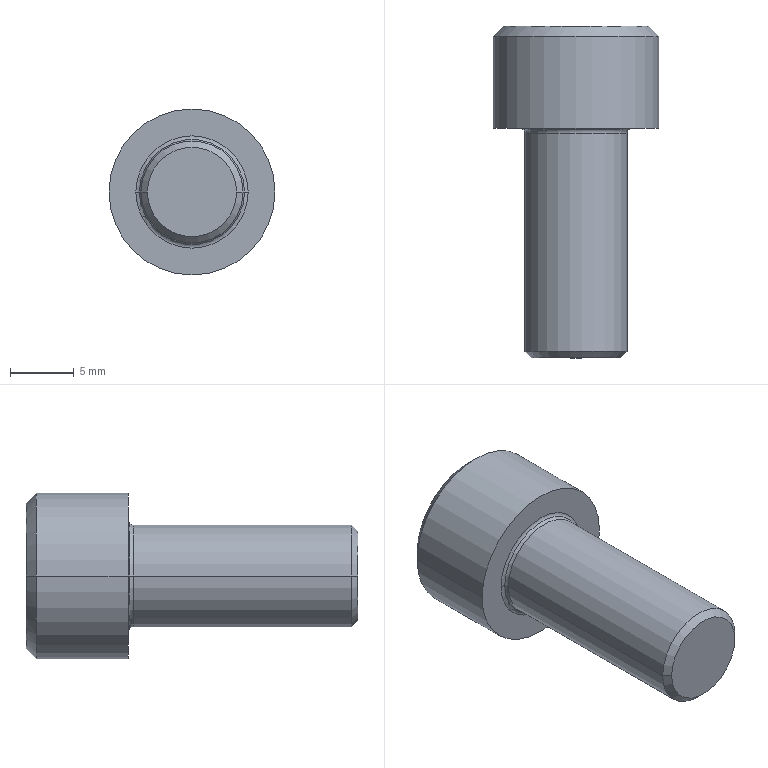Part | Creo | 1 solid | 23 faces | box 13 x 26 x 13 mm | volume 1803 mm3 | plane 9 | cone 6 | cylinder 4 | torus 4 | commonest cylinder face diameters 8 x2 13 x2
STEP:
#1=CARTESIAN_POINT('',(0.,0.,0.));
#2=DIRECTION('',(0.,0.,1.));
#3=DIRECTION('',(1.,0.,0.));
#4=AXIS2_PLACEMENT_3D('',#1,#2,#3);
#5=CARTESIAN_POINT('',(15.414,285.,18.42));
#6=VERTEX_POINT('',#5);
#7=CARTESIAN_POINT('',(13.682,285.,15.42));
#8=VERTEX_POINT('',#7);
#9=CARTESIAN_POINT('',(15.414,285.,18.42));
#10=CARTESIAN_POINT('',(15.371,284.975,18.344));
#11=CARTESIAN_POINT('',(15.285,284.928,18.196));
#12=CARTESIAN_POINT('',(15.161,284.87,17.981));
#13=CARTESIAN_POINT('',(15.039,284.821,17.771));
#14=CARTESIAN_POINT('',(14.918,284.782,17.561));
#15=CARTESIAN_POINT('',(14.796,284.754,17.349));
#16=CARTESIAN_POINT('',(14.673,284.736,17.135));
#17=CARTESIAN_POINT('',(14.548,284.73,16.92));
#18=CARTESIAN_POINT('',(14.424,284.736,16.704));
#19=CARTESIAN_POINT('',(14.3,284.754,16.49));
#20=CARTESIAN_POINT('',(14.178,284.782,16.278));
#21=CARTESIAN_POINT('',(14.057,284.821,16.069));
#22=CARTESIAN_POINT('',(13.935,284.87,15.858));
#23=CARTESIAN_POINT('',(13.811,284.928,15.643));
#24=CARTESIAN_POINT('',(13.726,284.975,15.495));
#25=CARTESIAN_POINT('',(13.682,285.,15.42));
#26=B_SPLINE_CURVE_WITH_KNOTS('',3,(#9,#10,#11,#12,#13,#14,#15,#16,#17,#18,#19,#20,#21,#22,#23,#24,#25),.UNSPECIFIED.,.F.,.F.,(4,1,1,1,1,1,1,1,1,1,1,1,1,1,4),(0.,0.07143,0.1429,0.2143,0.2857,0.3571,0.4286,0.5,0.5714,0.6429,0.7143,0.7857,0.8571,0.9286,1.),.UNSPECIFIED.);
#27=EDGE_CURVE('',#6,#8,#26,.T.);
#28=ORIENTED_EDGE('',*,*,#27,.F.);
#29=CARTESIAN_POINT('',(11.95,283.,18.42));
#30=VERTEX_POINT('',#29);
#31=CARTESIAN_POINT('',(11.95,283.,18.42));
#32=DIRECTION('',(0.866,0.5,0.));
#33=VECTOR('',#32,4.);
#34=LINE('',#31,#33);
#35=EDGE_CURVE('',#30,#6,#34,.T.);
#36=ORIENTED_EDGE('',*,*,#35,.F.);
#37=CARTESIAN_POINT('',(8.486,285.,18.42));
#38=VERTEX_POINT('',#37);
#39=CARTESIAN_POINT('',(11.95,283.,18.42));
#40=DIRECTION('',(-0.866,0.5,0.));
#41=VECTOR('',#40,4.);
#42=LINE('',#39,#41);
#43=EDGE_CURVE('',#30,#38,#42,.T.);
#44=ORIENTED_EDGE('',*,*,#43,.T.);
#45=CARTESIAN_POINT('',(10.218,285.,15.42));
#46=VERTEX_POINT('',#45);
#47=CARTESIAN_POINT('',(10.218,285.,15.42));
#48=CARTESIAN_POINT('',(10.174,284.975,15.495));
#49=CARTESIAN_POINT('',(10.089,284.928,15.643));
#50=CARTESIAN_POINT('',(9.965,284.87,15.858));
#51=CARTESIAN_POINT('',(9.843,284.821,16.069));
#52=CARTESIAN_POINT('',(9.722,284.782,16.278));
#53=CARTESIAN_POINT('',(9.6,284.754,16.49));
#54=CARTESIAN_POINT('',(9.476,284.736,16.704));
#55=CARTESIAN_POINT('',(9.352,284.73,16.92));
#56=CARTESIAN_POINT('',(9.227,284.736,17.135));
#57=CARTESIAN_POINT('',(9.104,284.754,17.349));
#58=CARTESIAN_POINT('',(8.982,284.782,17.561));
#59=CARTESIAN_POINT('',(8.861,284.821,17.771));
#60=CARTESIAN_POINT('',(8.739,284.87,17.981));
#61=CARTESIAN_POINT('',(8.615,284.928,18.196));
#62=CARTESIAN_POINT('',(8.529,284.975,18.344));
#63=CARTESIAN_POINT('',(8.486,285.,18.42));
#64=B_SPLINE_CURVE_WITH_KNOTS('',3,(#47,#48,#49,#50,#51,#52,#53,#54,#55,#56,#57,#58,#59,#60,#61,#62,#63),.UNSPECIFIED.,.F.,.F.,(4,1,1,1,1,1,1,1,1,1,1,1,1,1,4),(0.,0.07143,0.1429,0.2143,0.2857,0.3571,0.4286,0.5,0.5714,0.6429,0.7143,0.7857,0.8571,0.9286,1.),.UNSPECIFIED.);
#65=EDGE_CURVE('',#46,#38,#64,.T.);
#66=ORIENTED_EDGE('',*,*,#65,.F.);
#67=CARTESIAN_POINT('',(13.682,285.,15.42));
#68=CARTESIAN_POINT('',(13.595,284.975,15.42));
#69=CARTESIAN_POINT('',(13.424,284.928,15.42));
#70=CARTESIAN_POINT('',(13.177,284.87,15.42));
#71=CARTESIAN_POINT('',(12.934,284.821,15.42));
#72=CARTESIAN_POINT('',(12.692,284.782,15.42));
#73=CARTESIAN_POINT('',(12.447,284.754,15.42));
#74=CARTESIAN_POINT('',(12.199,284.736,15.42));
#75=CARTESIAN_POINT('',(11.95,284.73,15.42));
#76=CARTESIAN_POINT('',(11.701,284.736,15.42));
#77=CARTESIAN_POINT('',(11.453,284.754,15.42));
#78=CARTESIAN_POINT('',(11.208,284.782,15.42));
#79=CARTESIAN_POINT('',(10.966,284.821,15.42));
#80=CARTESIAN_POINT('',(10.723,284.87,15.42));
#81=CARTESIAN_POINT('',(10.476,284.928,15.42));
#82=CARTESIAN_POINT('',(10.305,284.975,15.42));
#83=CARTESIAN_POINT('',(10.218,285.,15.42));
#84=B_SPLINE_CURVE_WITH_KNOTS('',3,(#67,#68,#69,#70,#71,#72,#73,#74,#75,#76,#77,#78,#79,#80,#81,#82,#83),.UNSPECIFIED.,.F.,.F.,(4,1,1,1,1,1,1,1,1,1,1,1,1,1,4),(0.,0.07143,0.1429,0.2143,0.2857,0.3571,0.4286,0.5,0.5714,0.6429,0.7143,0.7857,0.8571,0.9286,1.),.UNSPECIFIED.);
#85=EDGE_CURVE('',#8,#46,#84,.T.);
#86=ORIENTED_EDGE('',*,*,#85,.F.);
#87=EDGE_LOOP('',(#28,#36,#44,#66,#86));
#88=FACE_OUTER_BOUND('',#87,.F.);
#89=CARTESIAN_POINT('',(11.95,284.02,18.42));
#90=DIRECTION('',(0.,1.,0.));
#91=DIRECTION('',(1.,0.,0.));
#92=AXIS2_PLACEMENT_3D('',#89,#90,#91);
#93=CONICAL_SURFACE('',#92,1.767,60.);
#94=ADVANCED_FACE('',(#88),#93,.F.);
#95=CARTESIAN_POINT('',(13.682,289.,15.42));
#96=VERTEX_POINT('',#95);
#97=CARTESIAN_POINT('',(15.414,289.,18.42));
#98=VERTEX_POINT('',#97);
#99=CARTESIAN_POINT('',(13.682,289.,15.42));
#100=DIRECTION('',(0.5,0.,0.866));
#101=VECTOR('',#100,3.464);
#102=LINE('',#99,#101);
#103=EDGE_CURVE('',#96,#98,#102,.T.);
#104=ORIENTED_EDGE('',*,*,#103,.T.);
#105=CARTESIAN_POINT('',(15.414,289.,18.42));
#106=DIRECTION('',(0.,-1.,0.));
#107=VECTOR('',#106,4.);
#108=LINE('',#105,#107);
#109=EDGE_CURVE('',#98,#6,#108,.T.);
#110=ORIENTED_EDGE('',*,*,#109,.T.);
#111=ORIENTED_EDGE('',*,*,#27,.T.);
#112=CARTESIAN_POINT('',(13.682,289.,15.42));
#113=DIRECTION('',(0.,-1.,0.));
#114=VECTOR('',#113,4.);
#115=LINE('',#112,#114);
#116=EDGE_CURVE('',#96,#8,#115,.T.);
#117=ORIENTED_EDGE('',*,*,#116,.F.);
#118=EDGE_LOOP('',(#104,#110,#111,#117));
#119=FACE_OUTER_BOUND('',#118,.F.);
#120=CARTESIAN_POINT('',(13.682,285.,15.42));
#121=DIRECTION('',(-0.866,0.,0.5));
#122=DIRECTION('',(0.5,0.,0.866));
#123=AXIS2_PLACEMENT_3D('',#120,#121,#122);
#124=PLANE('',#123);
#125=ADVANCED_FACE('',(#119),#124,.T.);
#126=CARTESIAN_POINT('',(17.65,289.,18.42));
#127=VERTEX_POINT('',#126);
#128=CARTESIAN_POINT('',(6.25,289.,18.42));
#129=VERTEX_POINT('',#128);
#130=CARTESIAN_POINT('',(11.95,289.,18.42));
#131=DIRECTION('',(0.,1.,0.));
#132=DIRECTION('',(1.,0.,0.));
#133=AXIS2_PLACEMENT_3D('',#130,#131,#132);
#134=CIRCLE('',#133,5.7);
#135=EDGE_CURVE('',#127,#129,#134,.T.);
#136=ORIENTED_EDGE('',*,*,#135,.F.);
#137=CARTESIAN_POINT('',(11.95,289.,18.42));
#138=DIRECTION('',(0.,1.,0.));
#139=DIRECTION('',(-1.,0.,0.));
#140=AXIS2_PLACEMENT_3D('',#137,#138,#139);
#141=CIRCLE('',#140,5.7);
#142=EDGE_CURVE('',#129,#127,#141,.T.);
#143=ORIENTED_EDGE('',*,*,#142,.F.);
#144=EDGE_LOOP('',(#136,#143));
#145=FACE_OUTER_BOUND('',#144,.F.);
#146=CARTESIAN_POINT('',(13.682,289.,21.42));
#147=VERTEX_POINT('',#146);
#148=CARTESIAN_POINT('',(15.414,289.,18.42));
#149=DIRECTION('',(-0.5,0.,0.866));
#150=VECTOR('',#149,3.464);
#151=LINE('',#148,#150);
#152=EDGE_CURVE('',#98,#147,#151,.T.);
#153=ORIENTED_EDGE('',*,*,#152,.F.);
#154=ORIENTED_EDGE('',*,*,#103,.F.);
#155=CARTESIAN_POINT('',(10.218,289.,15.42));
#156=VERTEX_POINT('',#155);
#157=CARTESIAN_POINT('',(13.682,289.,15.42));
#158=DIRECTION('',(-1.,0.,0.));
#159=VECTOR('',#158,3.464);
#160=LINE('',#157,#159);
#161=EDGE_CURVE('',#96,#156,#160,.T.);
#162=ORIENTED_EDGE('',*,*,#161,.T.);
#163=CARTESIAN_POINT('',(8.486,289.,18.42));
#164=VERTEX_POINT('',#163);
#165=CARTESIAN_POINT('',(8.486,289.,18.42));
#166=DIRECTION('',(0.5,0.,-0.866));
#167=VECTOR('',#166,3.464);
#168=LINE('',#165,#167);
#169=EDGE_CURVE('',#164,#156,#168,.T.);
#170=ORIENTED_EDGE('',*,*,#169,.F.);
#171=CARTESIAN_POINT('',(10.218,289.,21.42));
#172=VERTEX_POINT('',#171);
#173=CARTESIAN_POINT('',(10.218,289.,21.42));
#174=DIRECTION('',(-0.5,0.,-0.866));
#175=VECTOR('',#174,3.464);
#176=LINE('',#173,#175);
#177=EDGE_CURVE('',#172,#164,#176,.T.);
#178=ORIENTED_EDGE('',*,*,#177,.F.);
#179=CARTESIAN_POINT('',(10.218,289.,21.42));
#180=DIRECTION('',(1.,0.,0.));
#181=VECTOR('',#180,3.464);
#182=LINE('',#179,#181);
#183=EDGE_CURVE('',#172,#147,#182,.T.);
#184=ORIENTED_EDGE('',*,*,#183,.T.);
#185=EDGE_LOOP('',(#153,#154,#162,#170,#178,#184));
#186=FACE_BOUND('',#185,.F.);
#187=CARTESIAN_POINT('',(11.95,289.,18.42));
#188=DIRECTION('',(0.,1.,0.));
#189=DIRECTION('',(1.,0.,0.));
#190=AXIS2_PLACEMENT_3D('',#187,#188,#189);
#191=PLANE('',#190);
#192=ADVANCED_FACE('',(#145,#186),#191,.T.);
#193=CARTESIAN_POINT('',(18.45,288.2,18.42));
#194=VERTEX_POINT('',#193);
#195=CARTESIAN_POINT('',(5.45,288.2,18.42));
#196=VERTEX_POINT('',#195);
#197=CARTESIAN_POINT('',(11.95,288.2,18.42));
#198=DIRECTION('',(0.,1.,0.));
#199=DIRECTION('',(1.,0.,0.));
#200=AXIS2_PLACEMENT_3D('',#197,#198,#199);
#201=CIRCLE('',#200,6.5);
#202=EDGE_CURVE('',#194,#196,#201,.T.);
#203=ORIENTED_EDGE('',*,*,#202,.F.);
#204=CARTESIAN_POINT('',(17.65,289.,18.42));
#205=DIRECTION('',(0.7071,-0.7071,0.));
#206=VECTOR('',#205,1.131);
#207=LINE('',#204,#206);
#208=EDGE_CURVE('',#127,#194,#207,.T.);
#209=ORIENTED_EDGE('',*,*,#208,.F.);
#210=ORIENTED_EDGE('',*,*,#135,.T.);
#211=CARTESIAN_POINT('',(6.25,289.,18.42));
#212=DIRECTION('',(-0.7071,-0.7071,0.));
#213=VECTOR('',#212,1.131);
#214=LINE('',#211,#213);
#215=EDGE_CURVE('',#129,#196,#214,.T.);
#216=ORIENTED_EDGE('',*,*,#215,.T.);
#217=EDGE_LOOP('',(#203,#209,#210,#216));
#218=FACE_OUTER_BOUND('',#217,.F.);
#219=CARTESIAN_POINT('',(11.95,288.6,18.42));
#220=DIRECTION('',(0.,-1.,0.));
#221=DIRECTION('',(-1.,0.,0.));
#222=AXIS2_PLACEMENT_3D('',#219,#220,#221);
#223=CONICAL_SURFACE('',#222,6.1,45.);
#224=ADVANCED_FACE('',(#218),#223,.T.);
#225=ORIENTED_EDGE('',*,*,#202,.T.);
#226=CARTESIAN_POINT('',(5.45,281.,18.42));
#227=VERTEX_POINT('',#226);
#228=CARTESIAN_POINT('',(5.45,281.,18.42));
#229=DIRECTION('',(0.,1.,0.));
#230=VECTOR('',#229,7.2);
#231=LINE('',#228,#230);
#232=EDGE_CURVE('',#227,#196,#231,.T.);
#233=ORIENTED_EDGE('',*,*,#232,.F.);
#234=CARTESIAN_POINT('',(18.45,281.,18.42));
#235=VERTEX_POINT('',#234);
#236=CARTESIAN_POINT('',(11.95,281.,18.42));
#237=DIRECTION('',(0.,-1.,0.));
#238=DIRECTION('',(-1.,0.,0.));
#239=AXIS2_PLACEMENT_3D('',#236,#237,#238);
#240=CIRCLE('',#239,6.5);
#241=EDGE_CURVE('',#227,#235,#240,.T.);
#242=ORIENTED_EDGE('',*,*,#241,.T.);
#243=CARTESIAN_POINT('',(18.45,281.,18.42));
#244=DIRECTION('',(0.,1.,0.));
#245=VECTOR('',#244,7.2);
#246=LINE('',#243,#245);
#247=EDGE_CURVE('',#235,#194,#246,.T.);
#248=ORIENTED_EDGE('',*,*,#247,.T.);
#249=EDGE_LOOP('',(#225,#233,#242,#248));
#250=FACE_OUTER_BOUND('',#249,.F.);
#251=CARTESIAN_POINT('',(11.95,281.,18.42));
#252=DIRECTION('',(0.,1.,0.));
#253=DIRECTION('',(1.,0.,0.));
#254=AXIS2_PLACEMENT_3D('',#251,#252,#253);
#255=CYLINDRICAL_SURFACE('',#254,6.5);
#256=ADVANCED_FACE('',(#250),#255,.T.);
#257=CARTESIAN_POINT('',(11.95,288.2,18.42));
#258=DIRECTION('',(0.,1.,0.));
#259=DIRECTION('',(-1.,0.,0.));
#260=AXIS2_PLACEMENT_3D('',#257,#258,#259);
#261=CIRCLE('',#260,6.5);
#262=EDGE_CURVE('',#196,#194,#261,.T.);
#263=ORIENTED_EDGE('',*,*,#262,.T.);
#264=ORIENTED_EDGE('',*,*,#247,.F.);
#265=CARTESIAN_POINT('',(11.95,281.,18.42));
#266=DIRECTION('',(0.,-1.,0.));
#267=DIRECTION('',(1.,0.,0.));
#268=AXIS2_PLACEMENT_3D('',#265,#266,#267);
#269=CIRCLE('',#268,6.5);
#270=EDGE_CURVE('',#235,#227,#269,.T.);
#271=ORIENTED_EDGE('',*,*,#270,.T.);
#272=ORIENTED_EDGE('',*,*,#232,.T.);
#273=EDGE_LOOP('',(#263,#264,#271,#272));
#274=FACE_OUTER_BOUND('',#273,.F.);
#275=CARTESIAN_POINT('',(11.95,281.,18.42));
#276=DIRECTION('',(0.,1.,0.));
#277=DIRECTION('',(1.,0.,0.));
#278=AXIS2_PLACEMENT_3D('',#275,#276,#277);
#279=CYLINDRICAL_SURFACE('',#278,6.5);
#280=ADVANCED_FACE('',(#274),#279,.T.);
#281=ORIENTED_EDGE('',*,*,#262,.F.);
#282=ORIENTED_EDGE('',*,*,#215,.F.);
#283=ORIENTED_EDGE('',*,*,#142,.T.);
#284=ORIENTED_EDGE('',*,*,#208,.T.);
#285=EDGE_LOOP('',(#281,#282,#283,#284));
#286=FACE_OUTER_BOUND('',#285,.F.);
#287=CARTESIAN_POINT('',(11.95,288.6,18.42));
#288=DIRECTION('',(0.,-1.,0.));
#289=DIRECTION('',(-1.,0.,0.));
#290=AXIS2_PLACEMENT_3D('',#287,#288,#289);
#291=CONICAL_SURFACE('',#290,6.1,45.);
#292=ADVANCED_FACE('',(#286),#291,.T.);
#293=ORIENTED_EDGE('',*,*,#270,.F.);
#294=ORIENTED_EDGE('',*,*,#241,.F.);
#295=EDGE_LOOP('',(#293,#294));
#296=FACE_OUTER_BOUND('',#295,.F.);
#297=CARTESIAN_POINT('',(16.35,281.,18.42));
#298=VERTEX_POINT('',#297);
#299=CARTESIAN_POINT('',(7.55,281.,18.42));
#300=VERTEX_POINT('',#299);
#301=CARTESIAN_POINT('',(11.95,281.,18.42));
#302=DIRECTION('',(0.,1.,0.));
#303=DIRECTION('',(1.,0.,0.));
#304=AXIS2_PLACEMENT_3D('',#301,#302,#303);
#305=CIRCLE('',#304,4.4);
#306=EDGE_CURVE('',#298,#300,#305,.T.);
#307=ORIENTED_EDGE('',*,*,#306,.F.);
#308=CARTESIAN_POINT('',(11.95,281.,18.42));
#309=DIRECTION('',(0.,1.,0.));
#310=DIRECTION('',(-1.,0.,0.));
#311=AXIS2_PLACEMENT_3D('',#308,#309,#310);
#312=CIRCLE('',#311,4.4);
#313=EDGE_CURVE('',#300,#298,#312,.T.);
#314=ORIENTED_EDGE('',*,*,#313,.F.);
#315=EDGE_LOOP('',(#307,#314));
#316=FACE_BOUND('',#315,.F.);
#317=CARTESIAN_POINT('',(11.95,281.,18.42));
#318=DIRECTION('',(0.,1.,0.));
#319=DIRECTION('',(1.,0.,0.));
#320=AXIS2_PLACEMENT_3D('',#317,#318,#319);
#321=PLANE('',#320);
#322=ADVANCED_FACE('',(#296,#316),#321,.F.);
#323=ORIENTED_EDGE('',*,*,#306,.T.);
#324=CARTESIAN_POINT('',(7.833,280.883,18.42));
#325=VERTEX_POINT('',#324);
#326=CARTESIAN_POINT('',(7.55,280.6,18.42));
#327=DIRECTION('',(0.,0.,-1.));
#328=DIRECTION('',(0.,1.,0.));
#329=AXIS2_PLACEMENT_3D('',#326,#327,#328);
#330=CIRCLE('',#329,0.4);
#331=EDGE_CURVE('',#300,#325,#330,.T.);
#332=ORIENTED_EDGE('',*,*,#331,.T.);
#333=CARTESIAN_POINT('',(16.067,280.883,18.42));
#334=VERTEX_POINT('',#333);
#335=CARTESIAN_POINT('',(11.95,280.883,18.42));
#336=DIRECTION('',(0.,1.,0.));
#337=DIRECTION('',(1.,0.,0.));
#338=AXIS2_PLACEMENT_3D('',#335,#336,#337);
#339=CIRCLE('',#338,4.117);
#340=EDGE_CURVE('',#334,#325,#339,.T.);
#341=ORIENTED_EDGE('',*,*,#340,.F.);
#342=CARTESIAN_POINT('',(16.35,280.6,18.42));
#343=DIRECTION('',(0.,0.,1.));
#344=DIRECTION('',(0.,1.,0.));
#345=AXIS2_PLACEMENT_3D('',#342,#343,#344);
#346=CIRCLE('',#345,0.4);
#347=EDGE_CURVE('',#298,#334,#346,.T.);
#348=ORIENTED_EDGE('',*,*,#347,.F.);
#349=EDGE_LOOP('',(#323,#332,#341,#348));
#350=FACE_OUTER_BOUND('',#349,.F.);
#351=CARTESIAN_POINT('',(11.95,280.6,18.42));
#352=DIRECTION('',(0.,1.,0.));
#353=DIRECTION('',(1.,0.,0.));
#354=AXIS2_PLACEMENT_3D('',#351,#352,#353);
#355=TOROIDAL_SURFACE('',#354,4.4,0.4);
#356=ADVANCED_FACE('',(#350),#355,.F.);
#357=ORIENTED_EDGE('',*,*,#313,.T.);
#358=ORIENTED_EDGE('',*,*,#347,.T.);
#359=CARTESIAN_POINT('',(11.95,280.883,18.42));
#360=DIRECTION('',(0.,1.,0.));
#361=DIRECTION('',(-1.,0.,0.));
#362=AXIS2_PLACEMENT_3D('',#359,#360,#361);
#363=CIRCLE('',#362,4.117);
#364=EDGE_CURVE('',#325,#334,#363,.T.);
#365=ORIENTED_EDGE('',*,*,#364,.F.);
#366=ORIENTED_EDGE('',*,*,#331,.F.);
#367=EDGE_LOOP('',(#357,#358,#365,#366));
#368=FACE_OUTER_BOUND('',#367,.F.);
#369=CARTESIAN_POINT('',(11.95,280.6,18.42));
#370=DIRECTION('',(0.,1.,0.));
#371=DIRECTION('',(1.,0.,0.));
#372=AXIS2_PLACEMENT_3D('',#369,#370,#371);
#373=TOROIDAL_SURFACE('',#372,4.4,0.4);
#374=ADVANCED_FACE('',(#368),#373,.F.);
#375=CARTESIAN_POINT('',(7.95,280.6,18.42));
#376=VERTEX_POINT('',#375);
#377=CARTESIAN_POINT('',(15.95,280.6,18.42));
#378=VERTEX_POINT('',#377);
#379=CARTESIAN_POINT('',(11.95,280.6,18.42));
#380=DIRECTION('',(0.,1.,0.));
#381=DIRECTION('',(-1.,0.,0.));
#382=AXIS2_PLACEMENT_3D('',#379,#380,#381);
#383=CIRCLE('',#382,4.);
#384=EDGE_CURVE('',#376,#378,#383,.T.);
#385=ORIENTED_EDGE('',*,*,#384,.F.);
#386=CARTESIAN_POINT('',(7.55,280.6,18.42));
#387=DIRECTION('',(0.,0.,-1.));
#388=DIRECTION('',(0.7071,0.7071,0.));
#389=AXIS2_PLACEMENT_3D('',#386,#387,#388);
#390=CIRCLE('',#389,0.4);
#391=EDGE_CURVE('',#325,#376,#390,.T.);
#392=ORIENTED_EDGE('',*,*,#391,.F.);
#393=ORIENTED_EDGE('',*,*,#364,.T.);
#394=CARTESIAN_POINT('',(16.35,280.6,18.42));
#395=DIRECTION('',(0.,0.,1.));
#396=DIRECTION('',(-0.7071,0.7071,0.));
#397=AXIS2_PLACEMENT_3D('',#394,#395,#396);
#398=CIRCLE('',#397,0.4);
#399=EDGE_CURVE('',#334,#378,#398,.T.);
#400=ORIENTED_EDGE('',*,*,#399,.T.);
#401=EDGE_LOOP('',(#385,#392,#393,#400));
#402=FACE_OUTER_BOUND('',#401,.F.);
#403=CARTESIAN_POINT('',(11.95,280.6,18.42));
#404=DIRECTION('',(0.,1.,0.));
#405=DIRECTION('',(1.,0.,0.));
#406=AXIS2_PLACEMENT_3D('',#403,#404,#405);
#407=TOROIDAL_SURFACE('',#406,4.4,0.4);
#408=ADVANCED_FACE('',(#402),#407,.F.);
#409=CARTESIAN_POINT('',(15.95,263.5,18.42));
#410=VERTEX_POINT('',#409);
#411=CARTESIAN_POINT('',(7.95,263.5,18.42));
#412=VERTEX_POINT('',#411);
#413=CARTESIAN_POINT('',(11.95,263.5,18.42));
#414=DIRECTION('',(0.,-1.,0.));
#415=DIRECTION('',(1.,0.,0.));
#416=AXIS2_PLACEMENT_3D('',#413,#414,#415);
#417=CIRCLE('',#416,4.);
#418=EDGE_CURVE('',#410,#412,#417,.T.);
#419=ORIENTED_EDGE('',*,*,#418,.T.);
#420=CARTESIAN_POINT('',(7.95,263.5,18.42));
#421=DIRECTION('',(0.,1.,0.));
#422=VECTOR('',#421,17.1);
#423=LINE('',#420,#422);
#424=EDGE_CURVE('',#412,#376,#423,.T.);
#425=ORIENTED_EDGE('',*,*,#424,.T.);
#426=ORIENTED_EDGE('',*,*,#384,.T.);
#427=CARTESIAN_POINT('',(15.95,263.5,18.42));
#428=DIRECTION('',(0.,1.,0.));
#429=VECTOR('',#428,17.1);
#430=LINE('',#427,#429);
#431=EDGE_CURVE('',#410,#378,#430,.T.);
#432=ORIENTED_EDGE('',*,*,#431,.F.);
#433=EDGE_LOOP('',(#419,#425,#426,#432));
#434=FACE_OUTER_BOUND('',#433,.F.);
#435=CARTESIAN_POINT('',(11.95,263.,18.42));
#436=DIRECTION('',(0.,1.,0.));
#437=DIRECTION('',(1.,0.,0.));
#438=AXIS2_PLACEMENT_3D('',#435,#436,#437);
#439=CYLINDRICAL_SURFACE('',#438,4.);
#440=ADVANCED_FACE('',(#434),#439,.T.);
#441=CARTESIAN_POINT('',(15.45,263.,18.42));
#442=VERTEX_POINT('',#441);
#443=CARTESIAN_POINT('',(8.45,263.,18.42));
#444=VERTEX_POINT('',#443);
#445=CARTESIAN_POINT('',(11.95,263.,18.42));
#446=DIRECTION('',(0.,-1.,0.));
#447=DIRECTION('',(1.,0.,0.));
#448=AXIS2_PLACEMENT_3D('',#445,#446,#447);
#449=CIRCLE('',#448,3.5);
#450=EDGE_CURVE('',#442,#444,#449,.T.);
#451=ORIENTED_EDGE('',*,*,#450,.T.);
#452=CARTESIAN_POINT('',(8.45,263.,18.42));
#453=DIRECTION('',(-0.7071,0.7071,0.));
#454=VECTOR('',#453,0.7071);
#455=LINE('',#452,#454);
#456=EDGE_CURVE('',#444,#412,#455,.T.);
#457=ORIENTED_EDGE('',*,*,#456,.T.);
#458=ORIENTED_EDGE('',*,*,#418,.F.);
#459=CARTESIAN_POINT('',(15.45,263.,18.42));
#460=DIRECTION('',(0.7071,0.7071,0.));
#461=VECTOR('',#460,0.7071);
#462=LINE('',#459,#461);
#463=EDGE_CURVE('',#442,#410,#462,.T.);
#464=ORIENTED_EDGE('',*,*,#463,.F.);
#465=EDGE_LOOP('',(#451,#457,#458,#464));
#466=FACE_OUTER_BOUND('',#465,.F.);
#467=CARTESIAN_POINT('',(11.95,263.25,18.42));
#468=DIRECTION('',(0.,1.,0.));
#469=DIRECTION('',(1.,0.,0.));
#470=AXIS2_PLACEMENT_3D('',#467,#468,#469);
#471=CONICAL_SURFACE('',#470,3.75,45.);
#472=ADVANCED_FACE('',(#466),#471,.T.);
#473=ORIENTED_EDGE('',*,*,#450,.F.);
#474=CARTESIAN_POINT('',(11.95,263.,18.42));
#475=DIRECTION('',(0.,-1.,0.));
#476=DIRECTION('',(-1.,0.,0.));
#477=AXIS2_PLACEMENT_3D('',#474,#475,#476);
#478=CIRCLE('',#477,3.5);
#479=EDGE_CURVE('',#444,#442,#478,.T.);
#480=ORIENTED_EDGE('',*,*,#479,.F.);
#481=EDGE_LOOP('',(#473,#480));
#482=FACE_OUTER_BOUND('',#481,.F.);
#483=CARTESIAN_POINT('',(11.95,263.,18.42));
#484=DIRECTION('',(0.,1.,0.));
#485=DIRECTION('',(1.,0.,0.));
#486=AXIS2_PLACEMENT_3D('',#483,#484,#485);
#487=PLANE('',#486);
#488=ADVANCED_FACE('',(#482),#487,.F.);
#489=ORIENTED_EDGE('',*,*,#479,.T.);
#490=ORIENTED_EDGE('',*,*,#463,.T.);
#491=CARTESIAN_POINT('',(11.95,263.5,18.42));
#492=DIRECTION('',(0.,-1.,0.));
#493=DIRECTION('',(-1.,0.,0.));
#494=AXIS2_PLACEMENT_3D('',#491,#492,#493);
#495=CIRCLE('',#494,4.);
#496=EDGE_CURVE('',#412,#410,#495,.T.);
#497=ORIENTED_EDGE('',*,*,#496,.F.);
#498=ORIENTED_EDGE('',*,*,#456,.F.);
#499=EDGE_LOOP('',(#489,#490,#497,#498));
#500=FACE_OUTER_BOUND('',#499,.F.);
#501=CARTESIAN_POINT('',(11.95,263.25,18.42));
#502=DIRECTION('',(0.,1.,0.));
#503=DIRECTION('',(1.,0.,0.));
#504=AXIS2_PLACEMENT_3D('',#501,#502,#503);
#505=CONICAL_SURFACE('',#504,3.75,45.);
#506=ADVANCED_FACE('',(#500),#505,.T.);
#507=ORIENTED_EDGE('',*,*,#496,.T.);
#508=ORIENTED_EDGE('',*,*,#431,.T.);
#509=CARTESIAN_POINT('',(11.95,280.6,18.42));
#510=DIRECTION('',(0.,1.,0.));
#511=DIRECTION('',(1.,0.,0.));
#512=AXIS2_PLACEMENT_3D('',#509,#510,#511);
#513=CIRCLE('',#512,4.);
#514=EDGE_CURVE('',#378,#376,#513,.T.);
#515=ORIENTED_EDGE('',*,*,#514,.T.);
#516=ORIENTED_EDGE('',*,*,#424,.F.);
#517=EDGE_LOOP('',(#507,#508,#515,#516));
#518=FACE_OUTER_BOUND('',#517,.F.);
#519=CARTESIAN_POINT('',(11.95,263.,18.42));
#520=DIRECTION('',(0.,1.,0.));
#521=DIRECTION('',(1.,0.,0.));
#522=AXIS2_PLACEMENT_3D('',#519,#520,#521);
#523=CYLINDRICAL_SURFACE('',#522,4.);
#524=ADVANCED_FACE('',(#518),#523,.T.);
#525=ORIENTED_EDGE('',*,*,#514,.F.);
#526=ORIENTED_EDGE('',*,*,#399,.F.);
#527=ORIENTED_EDGE('',*,*,#340,.T.);
#528=ORIENTED_EDGE('',*,*,#391,.T.);
#529=EDGE_LOOP('',(#525,#526,#527,#528));
#530=FACE_OUTER_BOUND('',#529,.F.);
#531=CARTESIAN_POINT('',(11.95,280.6,18.42));
#532=DIRECTION('',(0.,1.,0.));
#533=DIRECTION('',(1.,0.,0.));
#534=AXIS2_PLACEMENT_3D('',#531,#532,#533);
#535=TOROIDAL_SURFACE('',#534,4.4,0.4);
#536=ADVANCED_FACE('',(#530),#535,.F.);
#537=ORIENTED_EDGE('',*,*,#152,.T.);
#538=CARTESIAN_POINT('',(13.682,285.,21.42));
#539=VERTEX_POINT('',#538);
#540=CARTESIAN_POINT('',(13.682,289.,21.42));
#541=DIRECTION('',(0.,-1.,0.));
#542=VECTOR('',#541,4.);
#543=LINE('',#540,#542);
#544=EDGE_CURVE('',#147,#539,#543,.T.);
#545=ORIENTED_EDGE('',*,*,#544,.T.);
#546=CARTESIAN_POINT('',(13.682,285.,21.42));
#547=CARTESIAN_POINT('',(13.726,284.975,21.344));
#548=CARTESIAN_POINT('',(13.811,284.928,21.196));
#549=CARTESIAN_POINT('',(13.935,284.87,20.981));
#550=CARTESIAN_POINT('',(14.057,284.821,20.771));
#551=CARTESIAN_POINT('',(14.178,284.782,20.561));
#552=CARTESIAN_POINT('',(14.3,284.754,20.349));
#553=CARTESIAN_POINT('',(14.424,284.736,20.135));
#554=CARTESIAN_POINT('',(14.548,284.73,19.92));
#555=CARTESIAN_POINT('',(14.673,284.736,19.704));
#556=CARTESIAN_POINT('',(14.796,284.754,19.49));
#557=CARTESIAN_POINT('',(14.918,284.782,19.278));
#558=CARTESIAN_POINT('',(15.039,284.821,19.069));
#559=CARTESIAN_POINT('',(15.161,284.87,18.858));
#560=CARTESIAN_POINT('',(15.285,284.928,18.643));
#561=CARTESIAN_POINT('',(15.371,284.975,18.495));
#562=CARTESIAN_POINT('',(15.414,285.,18.42));
#563=B_SPLINE_CURVE_WITH_KNOTS('',3,(#546,#547,#548,#549,#550,#551,#552,#553,#554,#555,#556,#557,#558,#559,#560,#561,#562),.UNSPECIFIED.,.F.,.F.,(4,1,1,1,1,1,1,1,1,1,1,1,1,1,4),(0.,0.07143,0.1429,0.2143,0.2857,0.3571,0.4286,0.5,0.5714,0.6429,0.7143,0.7857,0.8571,0.9286,1.),.UNSPECIFIED.);
#564=EDGE_CURVE('',#539,#6,#563,.T.);
#565=ORIENTED_EDGE('',*,*,#564,.T.);
#566=ORIENTED_EDGE('',*,*,#109,.F.);
#567=EDGE_LOOP('',(#537,#545,#565,#566));
#568=FACE_OUTER_BOUND('',#567,.F.);
#569=CARTESIAN_POINT('',(15.414,285.,18.42));
#570=DIRECTION('',(-0.866,0.,-0.5));
#571=DIRECTION('',(-0.5,0.,0.866));
#572=AXIS2_PLACEMENT_3D('',#569,#570,#571);
#573=PLANE('',#572);
#574=ADVANCED_FACE('',(#568),#573,.T.);
#575=ORIENTED_EDGE('',*,*,#183,.F.);
#576=CARTESIAN_POINT('',(10.218,285.,21.42));
#577=VERTEX_POINT('',#576);
#578=CARTESIAN_POINT('',(10.218,289.,21.42));
#579=DIRECTION('',(0.,-1.,0.));
#580=VECTOR('',#579,4.);
#581=LINE('',#578,#580);
#582=EDGE_CURVE('',#172,#577,#581,.T.);
#583=ORIENTED_EDGE('',*,*,#582,.T.);
#584=CARTESIAN_POINT('',(10.218,285.,21.42));
#585=CARTESIAN_POINT('',(10.305,284.975,21.42));
#586=CARTESIAN_POINT('',(10.476,284.928,21.42));
#587=CARTESIAN_POINT('',(10.723,284.87,21.42));
#588=CARTESIAN_POINT('',(10.966,284.821,21.42));
#589=CARTESIAN_POINT('',(11.208,284.782,21.42));
#590=CARTESIAN_POINT('',(11.453,284.754,21.42));
#591=CARTESIAN_POINT('',(11.701,284.736,21.42));
#592=CARTESIAN_POINT('',(11.95,284.73,21.42));
#593=CARTESIAN_POINT('',(12.199,284.736,21.42));
#594=CARTESIAN_POINT('',(12.447,284.754,21.42));
#595=CARTESIAN_POINT('',(12.692,284.782,21.42));
#596=CARTESIAN_POINT('',(12.934,284.821,21.42));
#597=CARTESIAN_POINT('',(13.177,284.87,21.42));
#598=CARTESIAN_POINT('',(13.424,284.928,21.42));
#599=CARTESIAN_POINT('',(13.595,284.975,21.42));
#600=CARTESIAN_POINT('',(13.682,285.,21.42));
#601=B_SPLINE_CURVE_WITH_KNOTS('',3,(#584,#585,#586,#587,#588,#589,#590,#591,#592,#593,#594,#595,#596,#597,#598,#599,#600),.UNSPECIFIED.,.F.,.F.,(4,1,1,1,1,1,1,1,1,1,1,1,1,1,4),(0.,0.07143,0.1429,0.2143,0.2857,0.3571,0.4286,0.5,0.5714,0.6429,0.7143,0.7857,0.8571,0.9286,1.),.UNSPECIFIED.);
#602=EDGE_CURVE('',#577,#539,#601,.T.);
#603=ORIENTED_EDGE('',*,*,#602,.T.);
#604=ORIENTED_EDGE('',*,*,#544,.F.);
#605=EDGE_LOOP('',(#575,#583,#603,#604));
#606=FACE_OUTER_BOUND('',#605,.F.);
#607=CARTESIAN_POINT('',(13.682,285.,21.42));
#608=DIRECTION('',(0.,0.,-1.));
#609=DIRECTION('',(0.,1.,0.));
#610=AXIS2_PLACEMENT_3D('',#607,#608,#609);
#611=PLANE('',#610);
#612=ADVANCED_FACE('',(#606),#611,.T.);
#613=ORIENTED_EDGE('',*,*,#177,.T.);
#614=CARTESIAN_POINT('',(8.486,289.,18.42));
#615=DIRECTION('',(0.,-1.,0.));
#616=VECTOR('',#615,4.);
#617=LINE('',#614,#616);
#618=EDGE_CURVE('',#164,#38,#617,.T.);
#619=ORIENTED_EDGE('',*,*,#618,.T.);
#620=CARTESIAN_POINT('',(8.486,285.,18.42));
#621=CARTESIAN_POINT('',(8.529,284.975,18.495));
#622=CARTESIAN_POINT('',(8.615,284.928,18.643));
#623=CARTESIAN_POINT('',(8.739,284.87,18.858));
#624=CARTESIAN_POINT('',(8.861,284.821,19.069));
#625=CARTESIAN_POINT('',(8.982,284.782,19.278));
#626=CARTESIAN_POINT('',(9.104,284.754,19.49));
#627=CARTESIAN_POINT('',(9.227,284.736,19.704));
#628=CARTESIAN_POINT('',(9.352,284.73,19.92));
#629=CARTESIAN_POINT('',(9.476,284.736,20.135));
#630=CARTESIAN_POINT('',(9.6,284.754,20.349));
#631=CARTESIAN_POINT('',(9.722,284.782,20.561));
#632=CARTESIAN_POINT('',(9.843,284.821,20.771));
#633=CARTESIAN_POINT('',(9.965,284.87,20.981));
#634=CARTESIAN_POINT('',(10.089,284.928,21.196));
#635=CARTESIAN_POINT('',(10.174,284.975,21.344));
#636=CARTESIAN_POINT('',(10.218,285.,21.42));
#637=B_SPLINE_CURVE_WITH_KNOTS('',3,(#620,#621,#622,#623,#624,#625,#626,#627,#628,#629,#630,#631,#632,#633,#634,#635,#636),.UNSPECIFIED.,.F.,.F.,(4,1,1,1,1,1,1,1,1,1,1,1,1,1,4),(0.,0.07143,0.1429,0.2143,0.2857,0.3571,0.4286,0.5,0.5714,0.6429,0.7143,0.7857,0.8571,0.9286,1.),.UNSPECIFIED.);
#638=EDGE_CURVE('',#38,#577,#637,.T.);
#639=ORIENTED_EDGE('',*,*,#638,.T.);
#640=ORIENTED_EDGE('',*,*,#582,.F.);
#641=EDGE_LOOP('',(#613,#619,#639,#640));
#642=FACE_OUTER_BOUND('',#641,.F.);
#643=CARTESIAN_POINT('',(10.218,285.,21.42));
#644=DIRECTION('',(0.866,0.,-0.5));
#645=DIRECTION('',(-0.5,0.,-0.866));
#646=AXIS2_PLACEMENT_3D('',#643,#644,#645);
#647=PLANE('',#646);
#648=ADVANCED_FACE('',(#642),#647,.T.);
#649=ORIENTED_EDGE('',*,*,#169,.T.);
#650=CARTESIAN_POINT('',(10.218,289.,15.42));
#651=DIRECTION('',(0.,-1.,0.));
#652=VECTOR('',#651,4.);
#653=LINE('',#650,#652);
#654=EDGE_CURVE('',#156,#46,#653,.T.);
#655=ORIENTED_EDGE('',*,*,#654,.T.);
#656=ORIENTED_EDGE('',*,*,#65,.T.);
#657=ORIENTED_EDGE('',*,*,#618,.F.);
#658=EDGE_LOOP('',(#649,#655,#656,#657));
#659=FACE_OUTER_BOUND('',#658,.F.);
#660=CARTESIAN_POINT('',(8.486,285.,18.42));
#661=DIRECTION('',(0.866,0.,0.5));
#662=DIRECTION('',(0.5,0.,-0.866));
#663=AXIS2_PLACEMENT_3D('',#660,#661,#662);
#664=PLANE('',#663);
#665=ADVANCED_FACE('',(#659),#664,.T.);
#666=ORIENTED_EDGE('',*,*,#161,.F.);
#667=ORIENTED_EDGE('',*,*,#116,.T.);
#668=ORIENTED_EDGE('',*,*,#85,.T.);
#669=ORIENTED_EDGE('',*,*,#654,.F.);
#670=EDGE_LOOP('',(#666,#667,#668,#669));
#671=FACE_OUTER_BOUND('',#670,.F.);
#672=CARTESIAN_POINT('',(10.218,285.,15.42));
#673=DIRECTION('',(0.,0.,1.));
#674=DIRECTION('',(0.,-1.,0.));
#675=AXIS2_PLACEMENT_3D('',#672,#673,#674);
#676=PLANE('',#675);
#677=ADVANCED_FACE('',(#671),#676,.T.);
#678=ORIENTED_EDGE('',*,*,#638,.F.);
#679=ORIENTED_EDGE('',*,*,#43,.F.);
#680=ORIENTED_EDGE('',*,*,#35,.T.);
#681=ORIENTED_EDGE('',*,*,#564,.F.);
#682=ORIENTED_EDGE('',*,*,#602,.F.);
#683=EDGE_LOOP('',(#678,#679,#680,#681,#682));
#684=FACE_OUTER_BOUND('',#683,.F.);
#685=CARTESIAN_POINT('',(11.95,284.02,18.42));
#686=DIRECTION('',(0.,1.,0.));
#687=DIRECTION('',(1.,0.,0.));
#688=AXIS2_PLACEMENT_3D('',#685,#686,#687);
#689=CONICAL_SURFACE('',#688,1.767,60.);
#690=ADVANCED_FACE('',(#684),#689,.F.);
#691=CLOSED_SHELL('',(#94,#125,#192,#224,#256,#280,#292,#322,#356,#374,#408,#440,#472,#488,#506,#524,#536,#574,#612,#648,#665,#677,#690));
#692=MANIFOLD_SOLID_BREP('',#691);
#693=(LENGTH_UNIT()NAMED_UNIT(*)SI_UNIT(.MILLI.,.METRE.));
#694=UNCERTAINTY_MEASURE_WITH_UNIT(LENGTH_MEASURE(0.003184),#693,'','');
#695=(NAMED_UNIT(*)PLANE_ANGLE_UNIT()SI_UNIT($,.RADIAN.));
#696=PLANE_ANGLE_MEASURE_WITH_UNIT(PLANE_ANGLE_MEASURE(0.01745),#695);
#697=(CONVERSION_BASED_UNIT('DEGREE',#696)NAMED_UNIT(*)PLANE_ANGLE_UNIT());
#698=(NAMED_UNIT(*)SI_UNIT($,.STERADIAN.)SOLID_ANGLE_UNIT());
#699=(GEOMETRIC_REPRESENTATION_CONTEXT(3)GLOBAL_UNCERTAINTY_ASSIGNED_CONTEXT((#694))GLOBAL_UNIT_ASSIGNED_CONTEXT((#693,#697,#698))REPRESENTATION_CONTEXT('',''));
#700=ADVANCED_BREP_SHAPE_REPRESENTATION('',(#4,#692),#699);